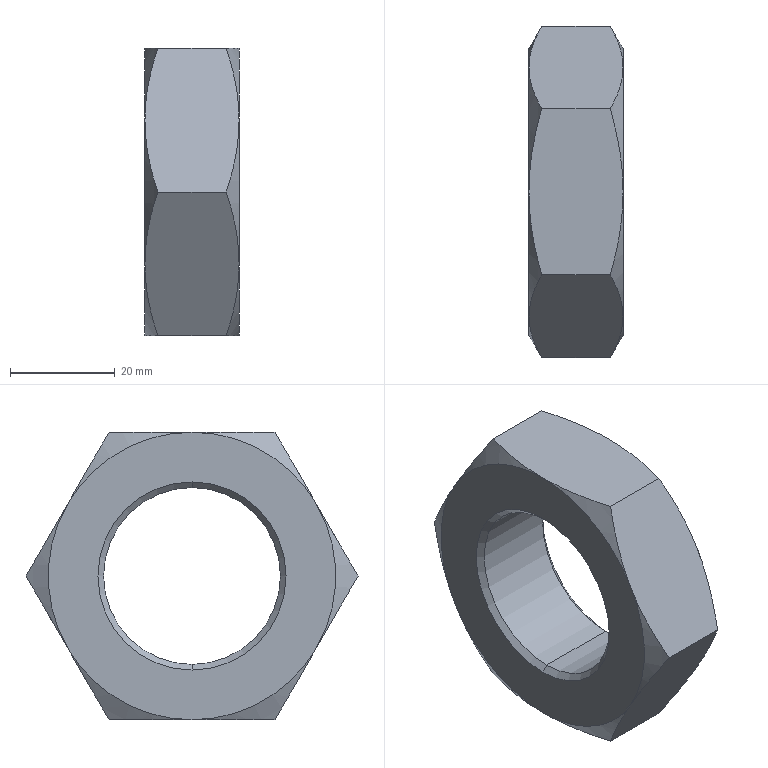Part | STEP file | 1 solid | 26 faces | box 18 x 63.509 x 55 mm | volume 30482 mm3 | cone 16 | plane 8 | cylinder 2 | commonest cylinder face diameters 33.835 x2